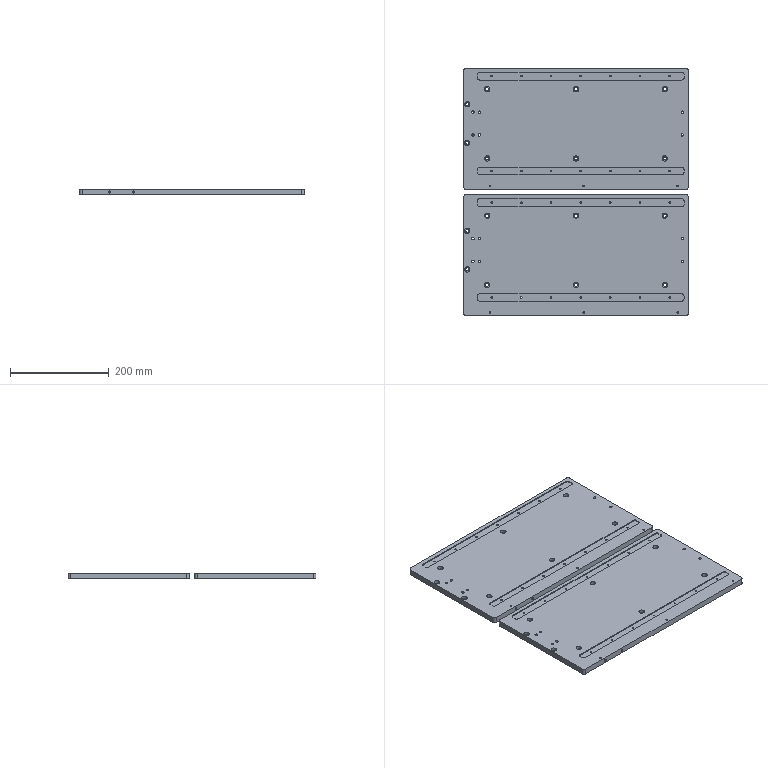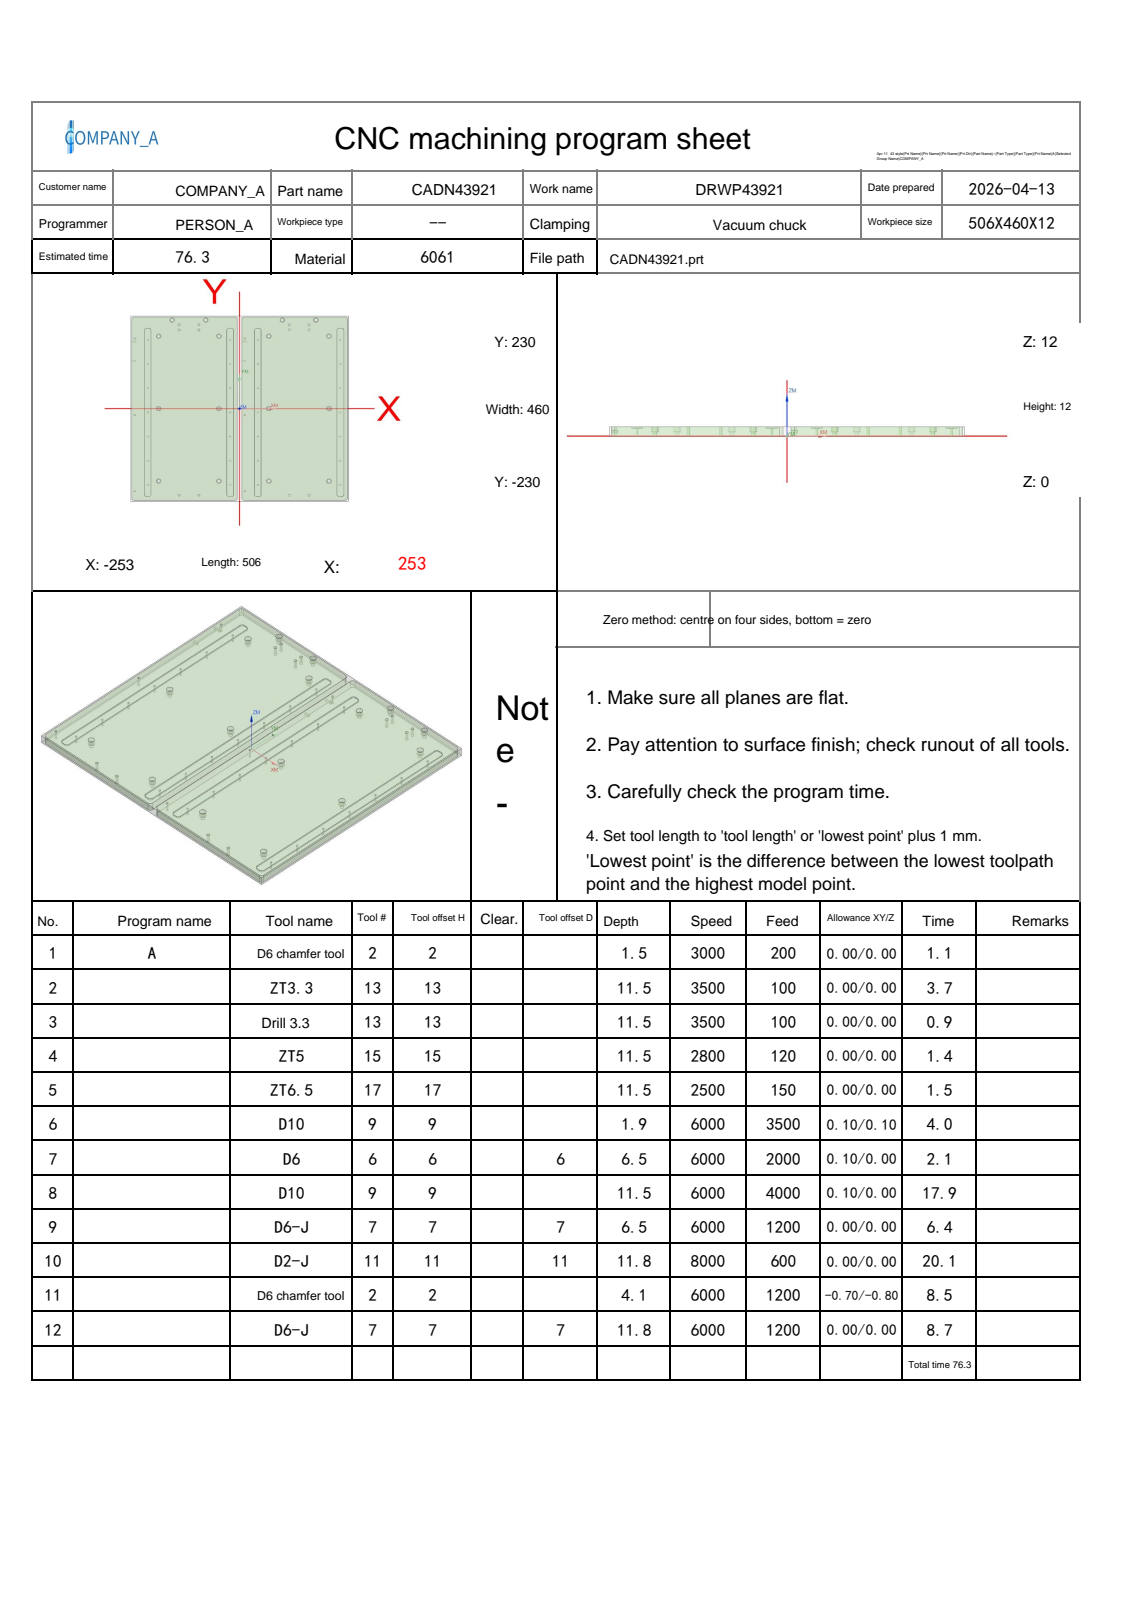NC program | NX | posted by the shop | part box 455 x 501 x 12 mm
Lines 1768 to 2613 of 11580:
N10 T11 M06
(D2-J  D=2. R=0. H=11 ce=0.00 di=0.00)
G00 G90 G54 X-190.045 Y179.151 M03 S8000
G43 H11 Z32.
M08
Z6.
G01 X-190.021 Y179.082 Z5.996 F600.
X-189.825 Y178.736 Z5.975
X-189.57 Y178.43 Z5.954
X-189.264 Y178.175 Z5.934
X-188.918 Y177.979 Z5.913
X-188.542 Y177.847 Z5.892
X-188.149 Y177.785 Z5.871
X-187.851 Z5.855
X-187.458 Y177.847 Z5.835
X-187.082 Y177.979 Z5.814
X-186.736 Y178.175 Z5.793
X-186.43 Y178.43 Z5.772
X-186.175 Y178.736 Z5.751
X-185.979 Y179.082 Z5.73
X-185.847 Y179.458 Z5.709
X-185.785 Y179.851 Z5.688
Y180.149 Z5.673
X-185.846 Y180.538 Z5.652
X-185.975 Y180.91 Z5.632
X-186.168 Y181.253 Z5.611
X-186.418 Y181.557 Z5.59
X-186.718 Y181.812 Z5.57
X-187.058 Y182.01 Z5.549
X-187.428 Y182.145 Z5.528
X-187.816 Y182.212 Z5.508
X-187.965 Y182.215 Z5.5
G41 D11
X-188. Y182.25
G03 X-190.25 Y180. Z5.417 I0.0 J-2.25
X-188. Y177.75 Z5.334 I2.25 J0.0
X-185.75 Y180. Z5.252 I0.0 J2.25
X-188. Y182.25 Z5.169 I-2.25 J0.0
X-190.25 Y180. Z5.086 I0.0 J-2.25
X-188. Y177.75 Z5.003 I2.25 J0.0
X-185.75 Y180. Z4.92 I0.0 J2.25
X-188. Y182.25 Z4.838 I-2.25 J0.0
X-190.25 Y180. Z4.755 I0.0 J-2.25
X-188. Y177.75 Z4.672 I2.25 J0.0
X-185.75 Y180. Z4.589 I0.0 J2.25
X-188. Y182.25 Z4.506 I-2.25 J0.0
X-190.25 Y180. Z4.423 I0.0 J-2.25
X-188. Y177.75 Z4.341 I2.25 J0.0
X-185.75 Y180. Z4.258 I0.0 J2.25
X-188. Y182.25 Z4.175 I-2.25 J0.0
X-190.25 Y180. Z4.092 I0.0 J-2.25
X-188. Y177.75 Z4.009 I2.25 J0.0
X-185.75 Y180. Z3.927 I0.0 J2.25
X-188. Y182.25 Z3.844 I-2.25 J0.0
X-190.25 Y180. Z3.761 I0.0 J-2.25
X-188. Y177.75 Z3.678 I2.25 J0.0
X-185.75 Y180. Z3.595 I0.0 J2.25
X-188. Y182.25 Z3.513 I-2.25 J0.0
X-190.25 Y180. Z3.43 I0.0 J-2.25
X-188. Y177.75 Z3.347 I2.25 J0.0
X-185.75 Y180. Z3.264 I0.0 J2.25
X-188. Y182.25 Z3.181 I-2.25 J0.0
X-190.25 Y180. Z3.098 I0.0 J-2.25
X-188. Y177.75 Z3.016 I2.25 J0.0
X-185.75 Y180. Z2.933 I0.0 J2.25
X-188. Y182.25 Z2.85 I-2.25 J0.0
X-190.25 Y180. Z2.767 I0.0 J-2.25
X-188. Y177.75 Z2.684 I2.25 J0.0
X-185.75 Y180. Z2.602 I0.0 J2.25
X-188. Y182.25 Z2.519 I-2.25 J0.0
X-190.25 Y180. Z2.436 I0.0 J-2.25
X-188. Y177.75 Z2.353 I2.25 J0.0
X-185.75 Y180. Z2.27 I0.0 J2.25
X-188. Y182.25 Z2.188 I-2.25 J0.0
X-190.25 Y180. Z2.105 I0.0 J-2.25
X-188. Y177.75 Z2.022 I2.25 J0.0
X-185.75 Y180. Z1.939 I0.0 J2.25
X-188. Y182.25 Z1.856 I-2.25 J0.0
X-190.25 Y180. Z1.773 I0.0 J-2.25
X-188. Y177.75 Z1.691 I2.25 J0.0
X-185.75 Y180. Z1.608 I0.0 J2.25
X-188. Y182.25 Z1.525 I-2.25 J0.0
X-190.25 Y180. Z1.442 I0.0 J-2.25
X-188. Y177.75 Z1.359 I2.25 J0.0
X-185.75 Y180. Z1.277 I0.0 J2.25
X-188. Y182.25 Z1.194 I-2.25 J0.0
X-190.25 Y180. Z1.111 I0.0 J-2.25
X-188. Y177.75 Z1.028 I2.25 J0.0
X-185.75 Y180. Z.945 I0.0 J2.25
X-188. Y182.25 Z.863 I-2.25 J0.0
X-190.25 Y180. Z.78 I0.0 J-2.25
X-188. Y177.75 Z.697 I2.25 J0.0
X-185.75 Y180. Z.614 I0.0 J2.25
X-188. Y182.25 Z.531 I-2.25 J0.0
X-190.25 Y180. Z.448 I0.0 J-2.25
X-188. Y177.75 Z.366 I2.25 J0.0
X-185.75 Y180. Z.283 I0.0 J2.25
X-188. Y182.25 Z.2 I-2.25 J0.0
X-190.25 Y180. I0.0 J-2.25
X-188. Y177.75 I2.25 J0.0
X-185.75 Y180. I0.0 J2.25
X-188. Y182.25 I-2.25 J0.0
X-188.398 Y182.215 I0.0 J-2.25
G01 X-188.425 Y182.207
X-188.441 Y182.184
X-188.438 Y182.156
G40 X-188.429 Y182.107
Z1.2
G00 Z32.
X-158.545 Y219.151
Z6.
G01 X-158.521 Y219.082 Z5.996
X-158.325 Y218.736 Z5.975
X-158.07 Y218.43 Z5.954
X-157.764 Y218.175 Z5.934
X-157.418 Y217.979 Z5.913
X-157.042 Y217.847 Z5.892
X-156.649 Y217.785 Z5.871
X-156.351 Z5.855
X-155.958 Y217.847 Z5.835
X-155.582 Y217.979 Z5.814
X-155.236 Y218.175 Z5.793
X-154.93 Y218.43 Z5.772
X-154.675 Y218.736 Z5.751
X-154.479 Y219.082 Z5.73
X-154.347 Y219.458 Z5.709
X-154.285 Y219.851 Z5.688
Y220.149 Z5.673
X-154.346 Y220.538 Z5.652
X-154.475 Y220.91 Z5.632
X-154.668 Y221.253 Z5.611
X-154.918 Y221.557 Z5.59
X-155.218 Y221.812 Z5.57
X-155.558 Y222.01 Z5.549
X-155.928 Y222.145 Z5.528
X-156.316 Y222.212 Z5.508
X-156.465 Y222.215 Z5.5
G41 D11
X-156.5 Y222.25
G03 X-158.75 Y220. Z5.417 I0.0 J-2.25
X-156.5 Y217.75 Z5.334 I2.25 J0.0
X-154.25 Y220. Z5.252 I0.0 J2.25
X-156.5 Y222.25 Z5.169 I-2.25 J0.0
X-158.75 Y220. Z5.086 I0.0 J-2.25
X-156.5 Y217.75 Z5.003 I2.25 J0.0
X-154.25 Y220. Z4.92 I0.0 J2.25
X-156.5 Y222.25 Z4.838 I-2.25 J0.0
X-158.75 Y220. Z4.755 I0.0 J-2.25
X-156.5 Y217.75 Z4.672 I2.25 J0.0
X-154.25 Y220. Z4.589 I0.0 J2.25
X-156.5 Y222.25 Z4.506 I-2.25 J0.0
X-158.75 Y220. Z4.423 I0.0 J-2.25
X-156.5 Y217.75 Z4.341 I2.25 J0.0
X-154.25 Y220. Z4.258 I0.0 J2.25
X-156.5 Y222.25 Z4.175 I-2.25 J0.0
X-158.75 Y220. Z4.092 I0.0 J-2.25
X-156.5 Y217.75 Z4.009 I2.25 J0.0
X-154.25 Y220. Z3.927 I0.0 J2.25
X-156.5 Y222.25 Z3.844 I-2.25 J0.0
X-158.75 Y220. Z3.761 I0.0 J-2.25
X-156.5 Y217.75 Z3.678 I2.25 J0.0
X-154.25 Y220. Z3.595 I0.0 J2.25
X-156.5 Y222.25 Z3.513 I-2.25 J0.0
X-158.75 Y220. Z3.43 I0.0 J-2.25
X-156.5 Y217.75 Z3.347 I2.25 J0.0
X-154.25 Y220. Z3.264 I0.0 J2.25
X-156.5 Y222.25 Z3.181 I-2.25 J0.0
X-158.75 Y220. Z3.098 I0.0 J-2.25
X-156.5 Y217.75 Z3.016 I2.25 J0.0
X-154.25 Y220. Z2.933 I0.0 J2.25
X-156.5 Y222.25 Z2.85 I-2.25 J0.0
X-158.75 Y220. Z2.767 I0.0 J-2.25
X-156.5 Y217.75 Z2.684 I2.25 J0.0
X-154.25 Y220. Z2.602 I0.0 J2.25
X-156.5 Y222.25 Z2.519 I-2.25 J0.0
X-158.75 Y220. Z2.436 I0.0 J-2.25
X-156.5 Y217.75 Z2.353 I2.25 J0.0
X-154.25 Y220. Z2.27 I0.0 J2.25
X-156.5 Y222.25 Z2.188 I-2.25 J0.0
X-158.75 Y220. Z2.105 I0.0 J-2.25
X-156.5 Y217.75 Z2.022 I2.25 J0.0
X-154.25 Y220. Z1.939 I0.0 J2.25
X-156.5 Y222.25 Z1.856 I-2.25 J0.0
X-158.75 Y220. Z1.773 I0.0 J-2.25
X-156.5 Y217.75 Z1.691 I2.25 J0.0
X-154.25 Y220. Z1.608 I0.0 J2.25
X-156.5 Y222.25 Z1.525 I-2.25 J0.0
X-158.75 Y220. Z1.442 I0.0 J-2.25
X-156.5 Y217.75 Z1.359 I2.25 J0.0
X-154.25 Y220. Z1.277 I0.0 J2.25
X-156.5 Y222.25 Z1.194 I-2.25 J0.0
X-158.75 Y220. Z1.111 I0.0 J-2.25
X-156.5 Y217.75 Z1.028 I2.25 J0.0
X-154.25 Y220. Z.945 I0.0 J2.25
X-156.5 Y222.25 Z.863 I-2.25 J0.0
X-158.75 Y220. Z.78 I0.0 J-2.25
X-156.5 Y217.75 Z.697 I2.25 J0.0
X-154.25 Y220. Z.614 I0.0 J2.25
X-156.5 Y222.25 Z.531 I-2.25 J0.0
X-158.75 Y220. Z.448 I0.0 J-2.25
X-156.5 Y217.75 Z.366 I2.25 J0.0
X-154.25 Y220. Z.283 I0.0 J2.25
X-156.5 Y222.25 Z.2 I-2.25 J0.0
X-158.75 Y220. I0.0 J-2.25
X-156.5 Y217.75 I2.25 J0.0
X-154.25 Y220. I0.0 J2.25
X-156.5 Y222.25 I-2.25 J0.0
X-156.898 Y222.215 I0.0 J-2.25
G01 X-156.925 Y222.207
X-156.941 Y222.184
X-156.938 Y222.156
G40 X-156.929 Y222.107
Z1.2
G00 Z32.
X-80.545 Y219.151
Z6.
G01 X-80.521 Y219.082 Z5.996
X-80.325 Y218.736 Z5.975
X-80.07 Y218.43 Z5.954
X-79.764 Y218.175 Z5.934
X-79.418 Y217.979 Z5.913
X-79.042 Y217.847 Z5.892
X-78.649 Y217.785 Z5.871
X-78.351 Z5.855
X-77.958 Y217.847 Z5.835
X-77.582 Y217.979 Z5.814
X-77.236 Y218.175 Z5.793
X-76.93 Y218.43 Z5.772
X-76.675 Y218.736 Z5.751
X-76.479 Y219.082 Z5.73
X-76.347 Y219.458 Z5.709
X-76.285 Y219.851 Z5.688
Y220.149 Z5.673
X-76.346 Y220.538 Z5.652
X-76.475 Y220.91 Z5.632
X-76.668 Y221.253 Z5.611
X-76.918 Y221.557 Z5.59
X-77.218 Y221.812 Z5.57
X-77.558 Y222.01 Z5.549
X-77.928 Y222.145 Z5.528
X-78.316 Y222.212 Z5.508
X-78.465 Y222.215 Z5.5
G41 D11
X-78.5 Y222.25
G03 X-80.75 Y220. Z5.417 I0.0 J-2.25
X-78.5 Y217.75 Z5.334 I2.25 J0.0
X-76.25 Y220. Z5.252 I0.0 J2.25
X-78.5 Y222.25 Z5.169 I-2.25 J0.0
X-80.75 Y220. Z5.086 I0.0 J-2.25
X-78.5 Y217.75 Z5.003 I2.25 J0.0
X-76.25 Y220. Z4.92 I0.0 J2.25
X-78.5 Y222.25 Z4.838 I-2.25 J0.0
X-80.75 Y220. Z4.755 I0.0 J-2.25
X-78.5 Y217.75 Z4.672 I2.25 J0.0
X-76.25 Y220. Z4.589 I0.0 J2.25
X-78.5 Y222.25 Z4.506 I-2.25 J0.0
X-80.75 Y220. Z4.423 I0.0 J-2.25
X-78.5 Y217.75 Z4.341 I2.25 J0.0
X-76.25 Y220. Z4.258 I0.0 J2.25
X-78.5 Y222.25 Z4.175 I-2.25 J0.0
X-80.75 Y220. Z4.092 I0.0 J-2.25
X-78.5 Y217.75 Z4.009 I2.25 J0.0
X-76.25 Y220. Z3.927 I0.0 J2.25
X-78.5 Y222.25 Z3.844 I-2.25 J0.0
X-80.75 Y220. Z3.761 I0.0 J-2.25
X-78.5 Y217.75 Z3.678 I2.25 J0.0
X-76.25 Y220. Z3.595 I0.0 J2.25
X-78.5 Y222.25 Z3.513 I-2.25 J0.0
X-80.75 Y220. Z3.43 I0.0 J-2.25
X-78.5 Y217.75 Z3.347 I2.25 J0.0
X-76.25 Y220. Z3.264 I0.0 J2.25
X-78.5 Y222.25 Z3.181 I-2.25 J0.0
X-80.75 Y220. Z3.098 I0.0 J-2.25
X-78.5 Y217.75 Z3.016 I2.25 J0.0
X-76.25 Y220. Z2.933 I0.0 J2.25
X-78.5 Y222.25 Z2.85 I-2.25 J0.0
X-80.75 Y220. Z2.767 I0.0 J-2.25
X-78.5 Y217.75 Z2.684 I2.25 J0.0
X-76.25 Y220. Z2.602 I0.0 J2.25
X-78.5 Y222.25 Z2.519 I-2.25 J0.0
X-80.75 Y220. Z2.436 I0.0 J-2.25
X-78.5 Y217.75 Z2.353 I2.25 J0.0
X-76.25 Y220. Z2.27 I0.0 J2.25
X-78.5 Y222.25 Z2.188 I-2.25 J0.0
X-80.75 Y220. Z2.105 I0.0 J-2.25
X-78.5 Y217.75 Z2.022 I2.25 J0.0
X-76.25 Y220. Z1.939 I0.0 J2.25
X-78.5 Y222.25 Z1.856 I-2.25 J0.0
X-80.75 Y220. Z1.773 I0.0 J-2.25
X-78.5 Y217.75 Z1.691 I2.25 J0.0
X-76.25 Y220. Z1.608 I0.0 J2.25
X-78.5 Y222.25 Z1.525 I-2.25 J0.0
X-80.75 Y220. Z1.442 I0.0 J-2.25
X-78.5 Y217.75 Z1.359 I2.25 J0.0
X-76.25 Y220. Z1.277 I0.0 J2.25
X-78.5 Y222.25 Z1.194 I-2.25 J0.0
X-80.75 Y220. Z1.111 I0.0 J-2.25
X-78.5 Y217.75 Z1.028 I2.25 J0.0
X-76.25 Y220. Z.945 I0.0 J2.25
X-78.5 Y222.25 Z.863 I-2.25 J0.0
X-80.75 Y220. Z.78 I0.0 J-2.25
X-78.5 Y217.75 Z.697 I2.25 J0.0
X-76.25 Y220. Z.614 I0.0 J2.25
X-78.5 Y222.25 Z.531 I-2.25 J0.0
X-80.75 Y220. Z.448 I0.0 J-2.25
X-78.5 Y217.75 Z.366 I2.25 J0.0
X-76.25 Y220. Z.283 I0.0 J2.25
X-78.5 Y222.25 Z.2 I-2.25 J0.0
X-80.75 Y220. I0.0 J-2.25
X-78.5 Y217.75 I2.25 J0.0
X-76.25 Y220. I0.0 J2.25
X-78.5 Y222.25 I-2.25 J0.0
X-78.898 Y222.215 I0.0 J-2.25
G01 X-78.925 Y222.207
X-78.941 Y222.184
X-78.938 Y222.156
G40 X-78.929 Y222.107
Z1.2
G00 Z32.
X-50.045 Y179.151
Z6.
G01 X-50.021 Y179.082 Z5.996
X-49.825 Y178.736 Z5.975
X-49.57 Y178.43 Z5.954
X-49.264 Y178.175 Z5.934
X-48.918 Y177.979 Z5.913
X-48.542 Y177.847 Z5.892
X-48.149 Y177.785 Z5.871
X-47.851 Z5.855
X-47.458 Y177.847 Z5.835
X-47.082 Y177.979 Z5.814
X-46.736 Y178.175 Z5.793
X-46.43 Y178.43 Z5.772
X-46.175 Y178.736 Z5.751
X-45.979 Y179.082 Z5.73
X-45.847 Y179.458 Z5.709
X-45.785 Y179.851 Z5.688
Y180.149 Z5.673
X-45.846 Y180.538 Z5.652
X-45.975 Y180.91 Z5.632
X-46.168 Y181.253 Z5.611
X-46.418 Y181.557 Z5.59
X-46.718 Y181.812 Z5.57
X-47.058 Y182.01 Z5.549
X-47.428 Y182.145 Z5.528
X-47.816 Y182.212 Z5.508
X-47.965 Y182.215 Z5.5
G41 D11
X-48. Y182.25
G03 X-50.25 Y180. Z5.417 I0.0 J-2.25
X-48. Y177.75 Z5.334 I2.25 J0.0
X-45.75 Y180. Z5.252 I0.0 J2.25
X-48. Y182.25 Z5.169 I-2.25 J0.0
X-50.25 Y180. Z5.086 I0.0 J-2.25
X-48. Y177.75 Z5.003 I2.25 J0.0
X-45.75 Y180. Z4.92 I0.0 J2.25
X-48. Y182.25 Z4.838 I-2.25 J0.0
X-50.25 Y180. Z4.755 I0.0 J-2.25
X-48. Y177.75 Z4.672 I2.25 J0.0
X-45.75 Y180. Z4.589 I0.0 J2.25
X-48. Y182.25 Z4.506 I-2.25 J0.0
X-50.25 Y180. Z4.423 I0.0 J-2.25
X-48. Y177.75 Z4.341 I2.25 J0.0
X-45.75 Y180. Z4.258 I0.0 J2.25
X-48. Y182.25 Z4.175 I-2.25 J0.0
X-50.25 Y180. Z4.092 I0.0 J-2.25
X-48. Y177.75 Z4.009 I2.25 J0.0
X-45.75 Y180. Z3.927 I0.0 J2.25
X-48. Y182.25 Z3.844 I-2.25 J0.0
X-50.25 Y180. Z3.761 I0.0 J-2.25
X-48. Y177.75 Z3.678 I2.25 J0.0
X-45.75 Y180. Z3.595 I0.0 J2.25
X-48. Y182.25 Z3.513 I-2.25 J0.0
X-50.25 Y180. Z3.43 I0.0 J-2.25
X-48. Y177.75 Z3.347 I2.25 J0.0
X-45.75 Y180. Z3.264 I0.0 J2.25
X-48. Y182.25 Z3.181 I-2.25 J0.0
X-50.25 Y180. Z3.098 I0.0 J-2.25
X-48. Y177.75 Z3.016 I2.25 J0.0
X-45.75 Y180. Z2.933 I0.0 J2.25
X-48. Y182.25 Z2.85 I-2.25 J0.0
X-50.25 Y180. Z2.767 I0.0 J-2.25
X-48. Y177.75 Z2.684 I2.25 J0.0
X-45.75 Y180. Z2.602 I0.0 J2.25
X-48. Y182.25 Z2.519 I-2.25 J0.0
X-50.25 Y180. Z2.436 I0.0 J-2.25
X-48. Y177.75 Z2.353 I2.25 J0.0
X-45.75 Y180. Z2.27 I0.0 J2.25
X-48. Y182.25 Z2.188 I-2.25 J0.0
X-50.25 Y180. Z2.105 I0.0 J-2.25
X-48. Y177.75 Z2.022 I2.25 J0.0
X-45.75 Y180. Z1.939 I0.0 J2.25
X-48. Y182.25 Z1.856 I-2.25 J0.0
X-50.25 Y180. Z1.773 I0.0 J-2.25
X-48. Y177.75 Z1.691 I2.25 J0.0
X-45.75 Y180. Z1.608 I0.0 J2.25
X-48. Y182.25 Z1.525 I-2.25 J0.0
X-50.25 Y180. Z1.442 I0.0 J-2.25
X-48. Y177.75 Z1.359 I2.25 J0.0
X-45.75 Y180. Z1.277 I0.0 J2.25
X-48. Y182.25 Z1.194 I-2.25 J0.0
X-50.25 Y180. Z1.111 I0.0 J-2.25
X-48. Y177.75 Z1.028 I2.25 J0.0
X-45.75 Y180. Z.945 I0.0 J2.25
X-48. Y182.25 Z.863 I-2.25 J0.0
X-50.25 Y180. Z.78 I0.0 J-2.25
X-48. Y177.75 Z.697 I2.25 J0.0
X-45.75 Y180. Z.614 I0.0 J2.25
X-48. Y182.25 Z.531 I-2.25 J0.0
X-50.25 Y180. Z.448 I0.0 J-2.25
X-48. Y177.75 Z.366 I2.25 J0.0
X-45.75 Y180. Z.283 I0.0 J2.25
X-48. Y182.25 Z.2 I-2.25 J0.0
X-50.25 Y180. I0.0 J-2.25
X-48. Y177.75 I2.25 J0.0
X-45.75 Y180. I0.0 J2.25
X-48. Y182.25 I-2.25 J0.0
X-48.398 Y182.215 I0.0 J-2.25
G01 X-48.425 Y182.207
X-48.441 Y182.184
X-48.438 Y182.156
G40 X-48.429 Y182.107
Z1.2
G00 Z32.
X65.955 Y179.151
Z6.
G01 X65.979 Y179.082 Z5.996
X66.175 Y178.736 Z5.975
X66.43 Y178.43 Z5.954
X66.736 Y178.175 Z5.934
X67.082 Y177.979 Z5.913
X67.458 Y177.847 Z5.892
X67.851 Y177.785 Z5.871
X68.149 Z5.855
X68.542 Y177.847 Z5.835
X68.918 Y177.979 Z5.814
X69.264 Y178.175 Z5.793
X69.57 Y178.43 Z5.772
X69.825 Y178.736 Z5.751
X70.021 Y179.082 Z5.73
X70.153 Y179.458 Z5.709
X70.215 Y179.851 Z5.688
Y180.149 Z5.673
X70.154 Y180.538 Z5.652
X70.025 Y180.91 Z5.632
X69.832 Y181.253 Z5.611
X69.582 Y181.557 Z5.59
X69.282 Y181.812 Z5.57
X68.942 Y182.01 Z5.549
X68.572 Y182.145 Z5.528
X68.184 Y182.212 Z5.508
X68.035 Y182.215 Z5.5
G41 D11
X68. Y182.25
G03 X65.75 Y180. Z5.417 I0.0 J-2.25
X68. Y177.75 Z5.334 I2.25 J0.0
X70.25 Y180. Z5.252 I0.0 J2.25
X68. Y182.25 Z5.169 I-2.25 J0.0
X65.75 Y180. Z5.086 I0.0 J-2.25
X68. Y177.75 Z5.003 I2.25 J0.0
X70.25 Y180. Z4.92 I0.0 J2.25
X68. Y182.25 Z4.838 I-2.25 J0.0
X65.75 Y180. Z4.755 I0.0 J-2.25
X68. Y177.75 Z4.672 I2.25 J0.0
X70.25 Y180. Z4.589 I0.0 J2.25
X68. Y182.25 Z4.506 I-2.25 J0.0
X65.75 Y180. Z4.423 I0.0 J-2.25
X68. Y177.75 Z4.341 I2.25 J0.0
X70.25 Y180. Z4.258 I0.0 J2.25
X68. Y182.25 Z4.175 I-2.25 J0.0
X65.75 Y180. Z4.092 I0.0 J-2.25
X68. Y177.75 Z4.009 I2.25 J0.0
X70.25 Y180. Z3.927 I0.0 J2.25
X68. Y182.25 Z3.844 I-2.25 J0.0
X65.75 Y180. Z3.761 I0.0 J-2.25
X68. Y177.75 Z3.678 I2.25 J0.0
X70.25 Y180. Z3.595 I0.0 J2.25
X68. Y182.25 Z3.513 I-2.25 J0.0
X65.75 Y180. Z3.43 I0.0 J-2.25
X68. Y177.75 Z3.347 I2.25 J0.0
X70.25 Y180. Z3.264 I0.0 J2.25
X68. Y182.25 Z3.181 I-2.25 J0.0
X65.75 Y180. Z3.098 I0.0 J-2.25
X68. Y177.75 Z3.016 I2.25 J0.0
X70.25 Y180. Z2.933 I0.0 J2.25
X68. Y182.25 Z2.85 I-2.25 J0.0
X65.75 Y180. Z2.767 I0.0 J-2.25
X68. Y177.75 Z2.684 I2.25 J0.0
X70.25 Y180. Z2.602 I0.0 J2.25
X68. Y182.25 Z2.519 I-2.25 J0.0
X65.75 Y180. Z2.436 I0.0 J-2.25
X68. Y177.75 Z2.353 I2.25 J0.0
X70.25 Y180. Z2.27 I0.0 J2.25
X68. Y182.25 Z2.188 I-2.25 J0.0
X65.75 Y180. Z2.105 I0.0 J-2.25
X68. Y177.75 Z2.022 I2.25 J0.0
X70.25 Y180. Z1.939 I0.0 J2.25
X68. Y182.25 Z1.856 I-2.25 J0.0
X65.75 Y180. Z1.773 I0.0 J-2.25
X68. Y177.75 Z1.691 I2.25 J0.0
X70.25 Y180. Z1.608 I0.0 J2.25
X68. Y182.25 Z1.525 I-2.25 J0.0
X65.75 Y180. Z1.442 I0.0 J-2.25
X68. Y177.75 Z1.359 I2.25 J0.0
X70.25 Y180. Z1.277 I0.0 J2.25
X68. Y182.25 Z1.194 I-2.25 J0.0
X65.75 Y180. Z1.111 I0.0 J-2.25
X68. Y177.75 Z1.028 I2.25 J0.0
X70.25 Y180. Z.945 I0.0 J2.25
X68. Y182.25 Z.863 I-2.25 J0.0
X65.75 Y180. Z.78 I0.0 J-2.25
X68. Y177.75 Z.697 I2.25 J0.0
X70.25 Y180. Z.614 I0.0 J2.25
X68. Y182.25 Z.531 I-2.25 J0.0
X65.75 Y180. Z.448 I0.0 J-2.25
X68. Y177.75 Z.366 I2.25 J0.0
X70.25 Y180. Z.283 I0.0 J2.25
X68. Y182.25 Z.2 I-2.25 J0.0
X65.75 Y180. I0.0 J-2.25
X68. Y177.75 I2.25 J0.0
X70.25 Y180. I0.0 J2.25
X68. Y182.25 I-2.25 J0.0
X67.602 Y182.215 I0.0 J-2.25
G01 X67.575 Y182.207
X67.559 Y182.184
X67.562 Y182.156
G40 X67.571 Y182.107
Z1.2
G00 Z32.
X97.455 Y219.151
Z6.
G01 X97.479 Y219.082 Z5.996
X97.675 Y218.736 Z5.975
X97.93 Y218.43 Z5.954
X98.236 Y218.175 Z5.934
X98.582 Y217.979 Z5.913
X98.958 Y217.847 Z5.892
X99.351 Y217.785 Z5.871
X99.649 Z5.855
X100.042 Y217.847 Z5.835
X100.418 Y217.979 Z5.814
X100.764 Y218.175 Z5.793
X101.07 Y218.43 Z5.772
X101.325 Y218.736 Z5.751
X101.521 Y219.082 Z5.73
X101.653 Y219.458 Z5.709
X101.715 Y219.851 Z5.688
Y220.149 Z5.673
X101.654 Y220.538 Z5.652
X101.525 Y220.91 Z5.632
X101.332 Y221.253 Z5.611
X101.082 Y221.557 Z5.59
X100.782 Y221.812 Z5.57
X100.442 Y222.01 Z5.549
X100.072 Y222.145 Z5.528
X99.684 Y222.212 Z5.508
X99.535 Y222.215 Z5.5
G41 D11
X99.5 Y222.25
G03 X97.25 Y220. Z5.417 I0.0 J-2.25
X99.5 Y217.75 Z5.334 I2.25 J0.0
X101.75 Y220. Z5.252 I0.0 J2.25
X99.5 Y222.25 Z5.169 I-2.25 J0.0
X97.25 Y220. Z5.086 I0.0 J-2.25
X99.5 Y217.75 Z5.003 I2.25 J0.0
X101.75 Y220. Z4.92 I0.0 J2.25
X99.5 Y222.25 Z4.838 I-2.25 J0.0
X97.25 Y220. Z4.755 I0.0 J-2.25
X99.5 Y217.75 Z4.672 I2.25 J0.0
X101.75 Y220. Z4.589 I0.0 J2.25
X99.5 Y222.25 Z4.506 I-2.25 J0.0
X97.25 Y220. Z4.423 I0.0 J-2.25
X99.5 Y217.75 Z4.341 I2.25 J0.0
X101.75 Y220. Z4.258 I0.0 J2.25
X99.5 Y222.25 Z4.175 I-2.25 J0.0
X97.25 Y220. Z4.092 I0.0 J-2.25
X99.5 Y217.75 Z4.009 I2.25 J0.0
X101.75 Y220. Z3.927 I0.0 J2.25
X99.5 Y222.25 Z3.844 I-2.25 J0.0
X97.25 Y220. Z3.761 I0.0 J-2.25
X99.5 Y217.75 Z3.678 I2.25 J0.0
X101.75 Y220. Z3.595 I0.0 J2.25
X99.5 Y222.25 Z3.513 I-2.25 J0.0
X97.25 Y220. Z3.43 I0.0 J-2.25
X99.5 Y217.75 Z3.347 I2.25 J0.0
X101.75 Y220. Z3.264 I0.0 J2.25
X99.5 Y222.25 Z3.181 I-2.25 J0.0
X97.25 Y220. Z3.098 I0.0 J-2.25
X99.5 Y217.75 Z3.016 I2.25 J0.0
X101.75 Y220. Z2.933 I0.0 J2.25
X99.5 Y222.25 Z2.85 I-2.25 J0.0
X97.25 Y220. Z2.767 I0.0 J-2.25
X99.5 Y217.75 Z2.684 I2.25 J0.0
X101.75 Y220. Z2.602 I0.0 J2.25
X99.5 Y222.25 Z2.519 I-2.25 J0.0
X97.25 Y220. Z2.436 I0.0 J-2.25
X99.5 Y217.75 Z2.353 I2.25 J0.0
X101.75 Y220. Z2.27 I0.0 J2.25
X99.5 Y222.25 Z2.188 I-2.25 J0.0
X97.25 Y220. Z2.105 I0.0 J-2.25
X99.5 Y217.75 Z2.022 I2.25 J0.0
X101.75 Y220. Z1.939 I0.0 J2.25
X99.5 Y222.25 Z1.856 I-2.25 J0.0
X97.25 Y220. Z1.773 I0.0 J-2.25
X99.5 Y217.75 Z1.691 I2.25 J0.0
X101.75 Y220. Z1.608 I0.0 J2.25
X99.5 Y222.25 Z1.525 I-2.25 J0.0
X97.25 Y220. Z1.442 I0.0 J-2.25
X99.5 Y217.75 Z1.359 I2.25 J0.0
X101.75 Y220. Z1.277 I0.0 J2.25
X99.5 Y222.25 Z1.194 I-2.25 J0.0
X97.25 Y220. Z1.111 I0.0 J-2.25
X99.5 Y217.75 Z1.028 I2.25 J0.0
X101.75 Y220. Z.945 I0.0 J2.25
X99.5 Y222.25 Z.863 I-2.25 J0.0
X97.25 Y220. Z.78 I0.0 J-2.25
X99.5 Y217.75 Z.697 I2.25 J0.0
X101.75 Y220. Z.614 I0.0 J2.25
X99.5 Y222.25 Z.531 I-2.25 J0.0
X97.25 Y220. Z.448 I0.0 J-2.25
X99.5 Y217.75 Z.366 I2.25 J0.0
X101.75 Y220. Z.283 I0.0 J2.25
X99.5 Y222.25 Z.2 I-2.25 J0.0
X97.25 Y220. I0.0 J-2.25
X99.5 Y217.75 I2.25 J0.0
X101.75 Y220. I0.0 J2.25
X99.5 Y222.25 I-2.25 J0.0
X99.102 Y222.215 I0.0 J-2.25
G01 X99.075 Y222.207
X99.059 Y222.184
X99.062 Y222.156
G40 X99.071 Y222.107
Z1.2
G00 Z32.
X175.455 Y219.151
Z6.
G01 X175.479 Y219.082 Z5.996
X175.675 Y218.736 Z5.975
X175.93 Y218.43 Z5.954
X176.236 Y218.175 Z5.934
X176.582 Y217.979 Z5.913
X176.958 Y217.847 Z5.892
X177.351 Y217.785 Z5.871
X177.649 Z5.855
X178.042 Y217.847 Z5.835
X178.418 Y217.979 Z5.814
X178.764 Y218.175 Z5.793
X179.07 Y218.43 Z5.772
X179.325 Y218.736 Z5.751
X179.521 Y219.082 Z5.73
X179.653 Y219.458 Z5.709
X179.715 Y219.851 Z5.688
Y220.149 Z5.673
X179.654 Y220.538 Z5.652
X179.525 Y220.91 Z5.632
X179.332 Y221.253 Z5.611
X179.082 Y221.557 Z5.59
X178.782 Y221.812 Z5.57
X178.442 Y222.01 Z5.549
X178.072 Y222.145 Z5.528
X177.684 Y222.212 Z5.508
X177.535 Y222.215 Z5.5
G41 D11
X177.5 Y222.25
G03 X175.25 Y220. Z5.417 I0.0 J-2.25
X177.5 Y217.75 Z5.334 I2.25 J0.0
X179.75 Y220. Z5.252 I0.0 J2.25
X177.5 Y222.25 Z5.169 I-2.25 J0.0
X175.25 Y220. Z5.086 I0.0 J-2.25
X177.5 Y217.75 Z5.003 I2.25 J0.0
X179.75 Y220. Z4.92 I0.0 J2.25
X177.5 Y222.25 Z4.838 I-2.25 J0.0
X175.25 Y220. Z4.755 I0.0 J-2.25
X177.5 Y217.75 Z4.672 I2.25 J0.0
X179.75 Y220. Z4.589 I0.0 J2.25
X177.5 Y222.25 Z4.506 I-2.25 J0.0
X175.25 Y220. Z4.423 I0.0 J-2.25
X177.5 Y217.75 Z4.341 I2.25 J0.0
X179.75 Y220. Z4.258 I0.0 J2.25
X177.5 Y222.25 Z4.175 I-2.25 J0.0
X175.25 Y220. Z4.092 I0.0 J-2.25
X177.5 Y217.75 Z4.009 I2.25 J0.0
X179.75 Y220. Z3.927 I0.0 J2.25
X177.5 Y222.25 Z3.844 I-2.25 J0.0
X175.25 Y220. Z3.761 I0.0 J-2.25
X177.5 Y217.75 Z3.678 I2.25 J0.0
X179.75 Y220. Z3.595 I0.0 J2.25
X177.5 Y222.25 Z3.513 I-2.25 J0.0
X175.25 Y220. Z3.43 I0.0 J-2.25
X177.5 Y217.75 Z3.347 I2.25 J0.0
X179.75 Y220. Z3.264 I0.0 J2.25
X177.5 Y222.25 Z3.181 I-2.25 J0.0
X175.25 Y220. Z3.098 I0.0 J-2.25
X177.5 Y217.75 Z3.016 I2.25 J0.0
X179.75 Y220. Z2.933 I0.0 J2.25
X177.5 Y222.25 Z2.85 I-2.25 J0.0
X175.25 Y220. Z2.767 I0.0 J-2.25
X177.5 Y217.75 Z2.684 I2.25 J0.0
X179.75 Y220. Z2.602 I0.0 J2.25
X177.5 Y222.25 Z2.519 I-2.25 J0.0
X175.25 Y220. Z2.436 I0.0 J-2.25
X177.5 Y217.75 Z2.353 I2.25 J0.0
X179.75 Y220. Z2.27 I0.0 J2.25
X177.5 Y222.25 Z2.188 I-2.25 J0.0
X175.25 Y220. Z2.105 I0.0 J-2.25
X177.5 Y217.75 Z2.022 I2.25 J0.0
X179.75 Y220. Z1.939 I0.0 J2.25
X177.5 Y222.25 Z1.856 I-2.25 J0.0
X175.25 Y220. Z1.773 I0.0 J-2.25
X177.5 Y217.75 Z1.691 I2.25 J0.0
X179.75 Y220. Z1.608 I0.0 J2.25
X177.5 Y222.25 Z1.525 I-2.25 J0.0
X175.25 Y220. Z1.442 I0.0 J-2.25
X177.5 Y217.75 Z1.359 I2.25 J0.0
X179.75 Y220. Z1.277 I0.0 J2.25
X177.5 Y222.25 Z1.194 I-2.25 J0.0
X175.25 Y220. Z1.111 I0.0 J-2.25
X177.5 Y217.75 Z1.028 I2.25 J0.0
X179.75 Y220. Z.945 I0.0 J2.25
X177.5 Y222.25 Z.863 I-2.25 J0.0
X175.25 Y220. Z.78 I0.0 J-2.25
X177.5 Y217.75 Z.697 I2.25 J0.0
X179.75 Y220. Z.614 I0.0 J2.25
X177.5 Y222.25 Z.531 I-2.25 J0.0
X175.25 Y220. Z.448 I0.0 J-2.25
X177.5 Y217.75 Z.366 I2.25 J0.0
X179.75 Y220. Z.283 I0.0 J2.25
X177.5 Y222.25 Z.2 I-2.25 J0.0
X175.25 Y220. I0.0 J-2.25
X177.5 Y217.75 I2.25 J0.0
X179.75 Y220. I0.0 J2.25
X177.5 Y222.25 I-2.25 J0.0
X177.102 Y222.215 I0.0 J-2.25
G01 X177.075 Y222.207
X177.059 Y222.184
X177.062 Y222.156
G40 X177.071 Y222.107
Z1.2
G00 Z32.
X207.151 Y182.045
Z6.
G01 X207.082 Y182.021 Z5.996
X206.736 Y181.825 Z5.975
X206.43 Y181.57 Z5.954
X206.175 Y181.264 Z5.934
X205.979 Y180.918 Z5.913
X205.847 Y180.542 Z5.892
X205.785 Y180.149 Z5.871
Y179.851 Z5.855
X205.847 Y179.458 Z5.835
X205.979 Y179.082 Z5.814
X206.175 Y178.736 Z5.793
X206.43 Y178.43 Z5.772
X206.736 Y178.175 Z5.751
X207.082 Y177.979 Z5.73
X207.458 Y177.847 Z5.709
X207.851 Y177.785 Z5.688
X208.149 Z5.673
X208.538 Y177.846 Z5.652
X208.91 Y177.975 Z5.632
X209.253 Y178.168 Z5.611
X209.557 Y178.418 Z5.59
X209.812 Y178.718 Z5.57
X210.01 Y179.058 Z5.549
X210.145 Y179.428 Z5.528
X210.212 Y179.816 Z5.508
X210.215 Y179.965 Z5.5
G41 D11
X210.25 Y180.
G03 X208. Y182.25 Z5.417 I-2.25 J0.0
X205.75 Y180. Z5.334 I0.0 J-2.25
X208. Y177.75 Z5.252 I2.25 J0.0
X210.25 Y180. Z5.169 I0.0 J2.25
X208. Y182.25 Z5.086 I-2.25 J0.0
X205.75 Y180. Z5.003 I0.0 J-2.25
X208. Y177.75 Z4.92 I2.25 J0.0
X210.25 Y180. Z4.838 I0.0 J2.25
X208. Y182.25 Z4.755 I-2.25 J0.0
X205.75 Y180. Z4.672 I0.0 J-2.25
X208. Y177.75 Z4.589 I2.25 J0.0
X210.25 Y180. Z4.506 I0.0 J2.25
X208. Y182.25 Z4.423 I-2.25 J0.0
X205.75 Y180. Z4.341 I0.0 J-2.25
X208. Y177.75 Z4.258 I2.25 J0.0
X210.25 Y180. Z4.175 I0.0 J2.25
X208. Y182.25 Z4.092 I-2.25 J0.0
X205.75 Y180. Z4.009 I0.0 J-2.25
X208. Y177.75 Z3.927 I2.25 J0.0
X210.25 Y180. Z3.844 I0.0 J2.25
X208. Y182.25 Z3.761 I-2.25 J0.0
X205.75 Y180. Z3.678 I0.0 J-2.25
X208. Y177.75 Z3.595 I2.25 J0.0
X210.25 Y180. Z3.513 I0.0 J2.25
X208. Y182.25 Z3.43 I-2.25 J0.0
X205.75 Y180. Z3.347 I0.0 J-2.25
X208. Y177.75 Z3.264 I2.25 J0.0
X210.25 Y180. Z3.181 I0.0 J2.25
X208. Y182.25 Z3.098 I-2.25 J0.0
X205.75 Y180. Z3.016 I0.0 J-2.25
X208. Y177.75 Z2.933 I2.25 J0.0
X210.25 Y180. Z2.85 I0.0 J2.25
X208. Y182.25 Z2.767 I-2.25 J0.0
X205.75 Y180. Z2.684 I0.0 J-2.25
X208. Y177.75 Z2.602 I2.25 J0.0
X210.25 Y180. Z2.519 I0.0 J2.25
X208. Y182.25 Z2.436 I-2.25 J0.0
X205.75 Y180. Z2.353 I0.0 J-2.25
X208. Y177.75 Z2.27 I2.25 J0.0
X210.25 Y180. Z2.188 I0.0 J2.25
X208. Y182.25 Z2.105 I-2.25 J0.0
X205.75 Y180. Z2.022 I0.0 J-2.25
X208. Y177.75 Z1.939 I2.25 J0.0
X210.25 Y180. Z1.856 I0.0 J2.25
X208. Y182.25 Z1.773 I-2.25 J0.0
X205.75 Y180. Z1.691 I0.0 J-2.25
X208. Y177.75 Z1.608 I2.25 J0.0
X210.25 Y180. Z1.525 I0.0 J2.25
X208. Y182.25 Z1.442 I-2.25 J0.0
X205.75 Y180. Z1.359 I0.0 J-2.25
X208. Y177.75 Z1.277 I2.25 J0.0
X210.25 Y180. Z1.194 I0.0 J2.25
X208. Y182.25 Z1.111 I-2.25 J0.0
X205.75 Y180. Z1.028 I0.0 J-2.25
X208. Y177.75 Z.945 I2.25 J0.0
X210.25 Y180. Z.863 I0.0 J2.25
X208. Y182.25 Z.78 I-2.25 J0.0
X205.75 Y180. Z.697 I0.0 J-2.25
X208. Y177.75 Z.614 I2.25 J0.0
X210.25 Y180. Z.531 I0.0 J2.25
X208. Y182.25 Z.448 I-2.25 J0.0
X205.75 Y180. Z.366 I0.0 J-2.25
X208. Y177.75 Z.283 I2.25 J0.0
X210.25 Y180. Z.2 I0.0 J2.25
X208. Y182.25 I-2.25 J0.0
X205.75 Y180. I0.0 J-2.25
X208. Y177.75 I2.25 J0.0
X210.25 Y180. I0.0 J2.25
X210.215 Y180.398 I-2.25 J0.0
G01 X210.207 Y180.425
X210.184 Y180.441
X210.156 Y180.438
G40 X210.107 Y180.429
Z1.2
G00 Z32.
X207.151 Y2.045
Z6.